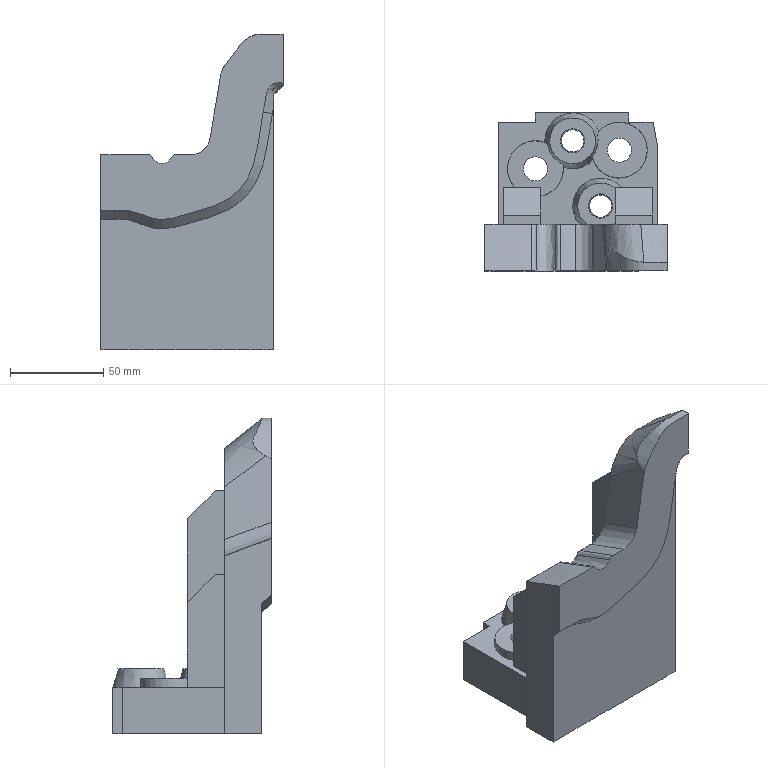Part | NX | features solid 2 | 1 solid | 58 faces | box 97.762 x 85 x 169.597 mm | volume 430121 mm3 | plane 32 | spline 14 | cylinder 9 | cone 3 | commonest cylinder face diameters 13 x4 30 x3 12 x2